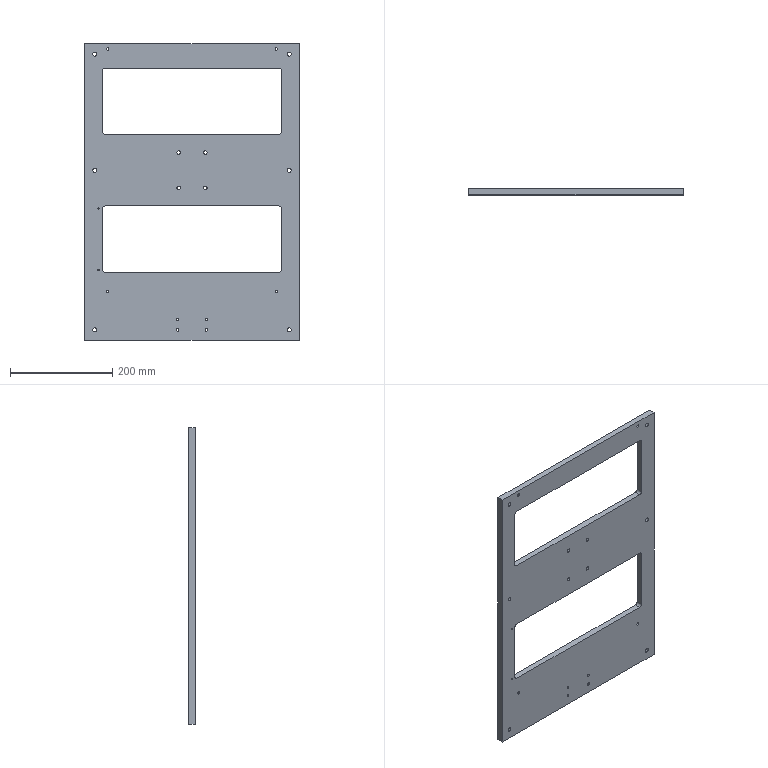Part | STEP file | 0230_201_Base | 1 solid | 62 faces | box 420 x 12 x 579.7 mm | volume 1822838 mm3 | cylinder 48 | plane 14 | commonest cylinder face diameters 5 x16 8 x12 6.8 x8 10 x8 2.5 x4